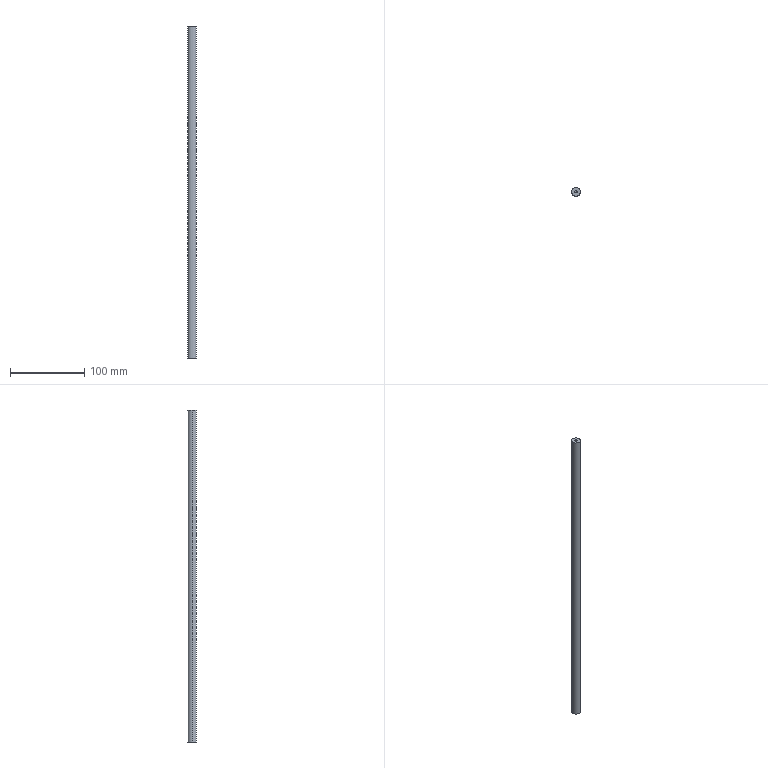Part | SolidWorks | features HoleWzd 2, Extrusion 1 | 1 solid | 12 faces | box 12 x 12 x 448 mm | volume 50405 mm3 | cylinder 6 | cone 4 | plane 2 | commonest cylinder face diameters 3.3 x4 12 x2
STEP:
#1=CARTESIAN_POINT('',(-1.65,0.,433.));
#2=VERTEX_POINT('',#1);
#3=CARTESIAN_POINT('',(1.65,0.,433.));
#4=VERTEX_POINT('',#3);
#5=CARTESIAN_POINT('',(0.,0.,433.));
#6=DIRECTION('',(0.,0.,1.));
#7=DIRECTION('',(1.,0.,0.));
#8=AXIS2_PLACEMENT_3D('',#5,#6,#7);
#9=CIRCLE('',#8,1.65);
#10=EDGE_CURVE('',#2,#4,#9,.T.);
#11=ORIENTED_EDGE('',*,*,#10,.F.);
#12=CARTESIAN_POINT('',(-1.65,0.,448.));
#13=VERTEX_POINT('',#12);
#14=CARTESIAN_POINT('',(-1.65,0.,448.));
#15=DIRECTION('',(0.,0.,1.));
#16=VECTOR('',#15,1000.);
#17=LINE('',#14,#16);
#18=EDGE_CURVE('',#2,#13,#17,.T.);
#19=ORIENTED_EDGE('',*,*,#18,.T.);
#20=CARTESIAN_POINT('',(1.65,0.,448.));
#21=VERTEX_POINT('',#20);
#22=CARTESIAN_POINT('',(0.,0.,448.));
#23=DIRECTION('',(0.,0.,1.));
#24=DIRECTION('',(1.,0.,0.));
#25=AXIS2_PLACEMENT_3D('',#22,#23,#24);
#26=CIRCLE('',#25,1.65);
#27=EDGE_CURVE('',#13,#21,#26,.T.);
#28=ORIENTED_EDGE('',*,*,#27,.T.);
#29=CARTESIAN_POINT('',(1.65,0.,448.));
#30=DIRECTION('',(0.,0.,1.));
#31=VECTOR('',#30,1000.);
#32=LINE('',#29,#31);
#33=EDGE_CURVE('',#4,#21,#32,.T.);
#34=ORIENTED_EDGE('',*,*,#33,.F.);
#35=EDGE_LOOP('',(#11,#19,#28,#34));
#36=FACE_OUTER_BOUND('',#35,.T.);
#37=CARTESIAN_POINT('',(0.,0.,448.));
#38=DIRECTION('',(0.,0.,1.));
#39=DIRECTION('',(1.,0.,0.));
#40=AXIS2_PLACEMENT_3D('',#37,#38,#39);
#41=CYLINDRICAL_SURFACE('',#40,1.65);
#42=ADVANCED_FACE('',(#36),#41,.F.);
#43=CARTESIAN_POINT('',(0.,0.,432.009));
#44=VERTEX_POINT('',#43);
#45=CARTESIAN_POINT('',(1.65,0.,433.));
#46=DIRECTION('',(0.8572,0.,0.515));
#47=VECTOR('',#46,1000.);
#48=LINE('',#45,#47);
#49=EDGE_CURVE('',#44,#4,#48,.T.);
#50=ORIENTED_EDGE('',*,*,#49,.F.);
#51=CARTESIAN_POINT('',(-1.65,0.,433.));
#52=DIRECTION('',(-0.8572,0.,0.515));
#53=VECTOR('',#52,1000.);
#54=LINE('',#51,#53);
#55=EDGE_CURVE('',#44,#2,#54,.T.);
#56=ORIENTED_EDGE('',*,*,#55,.T.);
#57=ORIENTED_EDGE('',*,*,#10,.T.);
#58=EDGE_LOOP('',(#50,#56,#57));
#59=FACE_OUTER_BOUND('',#58,.T.);
#60=CARTESIAN_POINT('',(0.,0.,433.));
#61=DIRECTION('',(0.,0.,1.));
#62=DIRECTION('',(1.,0.,0.));
#63=AXIS2_PLACEMENT_3D('',#60,#61,#62);
#64=CONICAL_SURFACE('',#63,1.65,1.03);
#65=ADVANCED_FACE('',(#59),#64,.F.);
#66=CARTESIAN_POINT('',(1.65,0.,15.));
#67=VERTEX_POINT('',#66);
#68=CARTESIAN_POINT('',(-1.65,0.,15.));
#69=VERTEX_POINT('',#68);
#70=CARTESIAN_POINT('',(0.,0.,15.));
#71=DIRECTION('',(0.,0.,-1.));
#72=DIRECTION('',(-1.,0.,0.));
#73=AXIS2_PLACEMENT_3D('',#70,#71,#72);
#74=CIRCLE('',#73,1.65);
#75=EDGE_CURVE('',#67,#69,#74,.T.);
#76=ORIENTED_EDGE('',*,*,#75,.F.);
#77=CARTESIAN_POINT('',(1.65,0.,0.));
#78=VERTEX_POINT('',#77);
#79=CARTESIAN_POINT('',(1.65,0.,0.));
#80=DIRECTION('',(0.,0.,-1.));
#81=VECTOR('',#80,1000.);
#82=LINE('',#79,#81);
#83=EDGE_CURVE('',#67,#78,#82,.T.);
#84=ORIENTED_EDGE('',*,*,#83,.T.);
#85=CARTESIAN_POINT('',(-1.65,0.,0.));
#86=VERTEX_POINT('',#85);
#87=CARTESIAN_POINT('',(0.,0.,0.));
#88=DIRECTION('',(0.,0.,-1.));
#89=DIRECTION('',(-1.,0.,0.));
#90=AXIS2_PLACEMENT_3D('',#87,#88,#89);
#91=CIRCLE('',#90,1.65);
#92=EDGE_CURVE('',#78,#86,#91,.T.);
#93=ORIENTED_EDGE('',*,*,#92,.T.);
#94=CARTESIAN_POINT('',(-1.65,0.,0.));
#95=DIRECTION('',(0.,0.,-1.));
#96=VECTOR('',#95,1000.);
#97=LINE('',#94,#96);
#98=EDGE_CURVE('',#69,#86,#97,.T.);
#99=ORIENTED_EDGE('',*,*,#98,.F.);
#100=EDGE_LOOP('',(#76,#84,#93,#99));
#101=FACE_OUTER_BOUND('',#100,.T.);
#102=CARTESIAN_POINT('',(0.,0.,0.));
#103=DIRECTION('',(0.,0.,-1.));
#104=DIRECTION('',(-1.,0.,0.));
#105=AXIS2_PLACEMENT_3D('',#102,#103,#104);
#106=CYLINDRICAL_SURFACE('',#105,1.65);
#107=ADVANCED_FACE('',(#101),#106,.F.);
#108=CARTESIAN_POINT('',(0.,0.,15.991));
#109=VERTEX_POINT('',#108);
#110=CARTESIAN_POINT('',(-1.65,0.,15.));
#111=DIRECTION('',(-0.8572,0.,-0.515));
#112=VECTOR('',#111,1000.);
#113=LINE('',#110,#112);
#114=EDGE_CURVE('',#109,#69,#113,.T.);
#115=ORIENTED_EDGE('',*,*,#114,.F.);
#116=CARTESIAN_POINT('',(1.65,0.,15.));
#117=DIRECTION('',(0.8572,0.,-0.515));
#118=VECTOR('',#117,1000.);
#119=LINE('',#116,#118);
#120=EDGE_CURVE('',#109,#67,#119,.T.);
#121=ORIENTED_EDGE('',*,*,#120,.T.);
#122=ORIENTED_EDGE('',*,*,#75,.T.);
#123=EDGE_LOOP('',(#115,#121,#122));
#124=FACE_OUTER_BOUND('',#123,.T.);
#125=CARTESIAN_POINT('',(0.,0.,15.));
#126=DIRECTION('',(0.,0.,-1.));
#127=DIRECTION('',(-1.,0.,0.));
#128=AXIS2_PLACEMENT_3D('',#125,#126,#127);
#129=CONICAL_SURFACE('',#128,1.65,1.03);
#130=ADVANCED_FACE('',(#124),#129,.F.);
#131=CARTESIAN_POINT('',(6.,0.,448.));
#132=VERTEX_POINT('',#131);
#133=CARTESIAN_POINT('',(-6.,0.,448.));
#134=VERTEX_POINT('',#133);
#135=CARTESIAN_POINT('',(0.,0.,448.));
#136=DIRECTION('',(0.,0.,1.));
#137=DIRECTION('',(1.,0.,0.));
#138=AXIS2_PLACEMENT_3D('',#135,#136,#137);
#139=CIRCLE('',#138,6.);
#140=EDGE_CURVE('',#132,#134,#139,.T.);
#141=ORIENTED_EDGE('',*,*,#140,.F.);
#142=CARTESIAN_POINT('',(6.,0.,0.));
#143=VERTEX_POINT('',#142);
#144=CARTESIAN_POINT('',(6.,0.,448.));
#145=DIRECTION('',(0.,0.,-1.));
#146=VECTOR('',#145,1000.);
#147=LINE('',#144,#146);
#148=EDGE_CURVE('',#132,#143,#147,.T.);
#149=ORIENTED_EDGE('',*,*,#148,.T.);
#150=CARTESIAN_POINT('',(-6.,0.,0.));
#151=VERTEX_POINT('',#150);
#152=CARTESIAN_POINT('',(0.,0.,0.));
#153=DIRECTION('',(0.,0.,1.));
#154=DIRECTION('',(1.,0.,0.));
#155=AXIS2_PLACEMENT_3D('',#152,#153,#154);
#156=CIRCLE('',#155,6.);
#157=EDGE_CURVE('',#143,#151,#156,.T.);
#158=ORIENTED_EDGE('',*,*,#157,.T.);
#159=CARTESIAN_POINT('',(-6.,0.,448.));
#160=DIRECTION('',(0.,0.,-1.));
#161=VECTOR('',#160,1000.);
#162=LINE('',#159,#161);
#163=EDGE_CURVE('',#134,#151,#162,.T.);
#164=ORIENTED_EDGE('',*,*,#163,.F.);
#165=EDGE_LOOP('',(#141,#149,#158,#164));
#166=FACE_OUTER_BOUND('',#165,.T.);
#167=CARTESIAN_POINT('',(0.,0.,448.));
#168=DIRECTION('',(0.,0.,-1.));
#169=DIRECTION('',(-1.,0.,0.));
#170=AXIS2_PLACEMENT_3D('',#167,#168,#169);
#171=CYLINDRICAL_SURFACE('',#170,6.);
#172=ADVANCED_FACE('',(#166),#171,.T.);
#173=ORIENTED_EDGE('',*,*,#148,.F.);
#174=CARTESIAN_POINT('',(0.,0.,448.));
#175=DIRECTION('',(0.,0.,1.));
#176=DIRECTION('',(1.,0.,0.));
#177=AXIS2_PLACEMENT_3D('',#174,#175,#176);
#178=CIRCLE('',#177,6.);
#179=EDGE_CURVE('',#134,#132,#178,.T.);
#180=ORIENTED_EDGE('',*,*,#179,.F.);
#181=ORIENTED_EDGE('',*,*,#163,.T.);
#182=CARTESIAN_POINT('',(0.,0.,0.));
#183=DIRECTION('',(0.,0.,1.));
#184=DIRECTION('',(1.,0.,0.));
#185=AXIS2_PLACEMENT_3D('',#182,#183,#184);
#186=CIRCLE('',#185,6.);
#187=EDGE_CURVE('',#151,#143,#186,.T.);
#188=ORIENTED_EDGE('',*,*,#187,.T.);
#189=EDGE_LOOP('',(#173,#180,#181,#188));
#190=FACE_OUTER_BOUND('',#189,.T.);
#191=CARTESIAN_POINT('',(0.,0.,448.));
#192=DIRECTION('',(0.,0.,-1.));
#193=DIRECTION('',(-1.,0.,0.));
#194=AXIS2_PLACEMENT_3D('',#191,#192,#193);
#195=CYLINDRICAL_SURFACE('',#194,6.);
#196=ADVANCED_FACE('',(#190),#195,.T.);
#197=CARTESIAN_POINT('',(0.,0.,448.));
#198=DIRECTION('',(0.,0.,1.));
#199=DIRECTION('',(1.,0.,0.));
#200=AXIS2_PLACEMENT_3D('',#197,#198,#199);
#201=CIRCLE('',#200,1.65);
#202=EDGE_CURVE('',#21,#13,#201,.T.);
#203=ORIENTED_EDGE('',*,*,#202,.F.);
#204=ORIENTED_EDGE('',*,*,#27,.F.);
#205=EDGE_LOOP('',(#203,#204));
#206=FACE_BOUND('',#205,.T.);
#207=ORIENTED_EDGE('',*,*,#179,.T.);
#208=ORIENTED_EDGE('',*,*,#140,.T.);
#209=EDGE_LOOP('',(#207,#208));
#210=FACE_OUTER_BOUND('',#209,.T.);
#211=CARTESIAN_POINT('',(0.,0.,448.));
#212=DIRECTION('',(0.,0.,1.));
#213=DIRECTION('',(1.,0.,0.));
#214=AXIS2_PLACEMENT_3D('',#211,#212,#213);
#215=PLANE('',#214);
#216=ADVANCED_FACE('',(#206,#210),#215,.T.);
#217=CARTESIAN_POINT('',(0.,0.,0.));
#218=DIRECTION('',(0.,0.,-1.));
#219=DIRECTION('',(-1.,0.,0.));
#220=AXIS2_PLACEMENT_3D('',#217,#218,#219);
#221=CIRCLE('',#220,1.65);
#222=EDGE_CURVE('',#86,#78,#221,.T.);
#223=ORIENTED_EDGE('',*,*,#222,.F.);
#224=ORIENTED_EDGE('',*,*,#92,.F.);
#225=EDGE_LOOP('',(#223,#224));
#226=FACE_BOUND('',#225,.T.);
#227=ORIENTED_EDGE('',*,*,#187,.F.);
#228=ORIENTED_EDGE('',*,*,#157,.F.);
#229=EDGE_LOOP('',(#227,#228));
#230=FACE_OUTER_BOUND('',#229,.T.);
#231=CARTESIAN_POINT('',(0.,0.,0.));
#232=DIRECTION('',(0.,0.,1.));
#233=DIRECTION('',(1.,0.,0.));
#234=AXIS2_PLACEMENT_3D('',#231,#232,#233);
#235=PLANE('',#234);
#236=ADVANCED_FACE('',(#226,#230),#235,.F.);
#237=ORIENTED_EDGE('',*,*,#120,.F.);
#238=ORIENTED_EDGE('',*,*,#114,.T.);
#239=CARTESIAN_POINT('',(0.,0.,15.));
#240=DIRECTION('',(0.,0.,-1.));
#241=DIRECTION('',(-1.,0.,0.));
#242=AXIS2_PLACEMENT_3D('',#239,#240,#241);
#243=CIRCLE('',#242,1.65);
#244=EDGE_CURVE('',#69,#67,#243,.T.);
#245=ORIENTED_EDGE('',*,*,#244,.T.);
#246=EDGE_LOOP('',(#237,#238,#245));
#247=FACE_OUTER_BOUND('',#246,.T.);
#248=CARTESIAN_POINT('',(0.,0.,15.));
#249=DIRECTION('',(0.,0.,-1.));
#250=DIRECTION('',(-1.,0.,0.));
#251=AXIS2_PLACEMENT_3D('',#248,#249,#250);
#252=CONICAL_SURFACE('',#251,1.65,1.03);
#253=ADVANCED_FACE('',(#247),#252,.F.);
#254=ORIENTED_EDGE('',*,*,#83,.F.);
#255=ORIENTED_EDGE('',*,*,#244,.F.);
#256=ORIENTED_EDGE('',*,*,#98,.T.);
#257=ORIENTED_EDGE('',*,*,#222,.T.);
#258=EDGE_LOOP('',(#254,#255,#256,#257));
#259=FACE_OUTER_BOUND('',#258,.T.);
#260=CARTESIAN_POINT('',(0.,0.,0.));
#261=DIRECTION('',(0.,0.,-1.));
#262=DIRECTION('',(-1.,0.,0.));
#263=AXIS2_PLACEMENT_3D('',#260,#261,#262);
#264=CYLINDRICAL_SURFACE('',#263,1.65);
#265=ADVANCED_FACE('',(#259),#264,.F.);
#266=ORIENTED_EDGE('',*,*,#55,.F.);
#267=ORIENTED_EDGE('',*,*,#49,.T.);
#268=CARTESIAN_POINT('',(0.,0.,433.));
#269=DIRECTION('',(0.,0.,1.));
#270=DIRECTION('',(1.,0.,0.));
#271=AXIS2_PLACEMENT_3D('',#268,#269,#270);
#272=CIRCLE('',#271,1.65);
#273=EDGE_CURVE('',#4,#2,#272,.T.);
#274=ORIENTED_EDGE('',*,*,#273,.T.);
#275=EDGE_LOOP('',(#266,#267,#274));
#276=FACE_OUTER_BOUND('',#275,.T.);
#277=CARTESIAN_POINT('',(0.,0.,433.));
#278=DIRECTION('',(0.,0.,1.));
#279=DIRECTION('',(1.,0.,0.));
#280=AXIS2_PLACEMENT_3D('',#277,#278,#279);
#281=CONICAL_SURFACE('',#280,1.65,1.03);
#282=ADVANCED_FACE('',(#276),#281,.F.);
#283=ORIENTED_EDGE('',*,*,#18,.F.);
#284=ORIENTED_EDGE('',*,*,#273,.F.);
#285=ORIENTED_EDGE('',*,*,#33,.T.);
#286=ORIENTED_EDGE('',*,*,#202,.T.);
#287=EDGE_LOOP('',(#283,#284,#285,#286));
#288=FACE_OUTER_BOUND('',#287,.T.);
#289=CARTESIAN_POINT('',(0.,0.,448.));
#290=DIRECTION('',(0.,0.,1.));
#291=DIRECTION('',(1.,0.,0.));
#292=AXIS2_PLACEMENT_3D('',#289,#290,#291);
#293=CYLINDRICAL_SURFACE('',#292,1.65);
#294=ADVANCED_FACE('',(#288),#293,.F.);
#295=CLOSED_SHELL('',(#42,#65,#107,#130,#172,#196,#216,#236,#253,#265,#282,#294));
#296=MANIFOLD_SOLID_BREP('',#295);
#297=CARTESIAN_POINT('',(0.,0.,0.));
#298=DIRECTION('',(0.,0.,1.));
#299=DIRECTION('',(1.,0.,0.));
#300=AXIS2_PLACEMENT_3D('',#297,#298,#299);
#301=(LENGTH_UNIT()NAMED_UNIT(*)SI_UNIT(.MILLI.,.METRE.));
#302=UNCERTAINTY_MEASURE_WITH_UNIT(LENGTH_MEASURE(0.00001),#301,'','');
#303=(NAMED_UNIT(*)PLANE_ANGLE_UNIT()SI_UNIT($,.RADIAN.));
#304=(NAMED_UNIT(*)SI_UNIT($,.STERADIAN.)SOLID_ANGLE_UNIT());
#305=(GEOMETRIC_REPRESENTATION_CONTEXT(3)GLOBAL_UNCERTAINTY_ASSIGNED_CONTEXT((#302))GLOBAL_UNIT_ASSIGNED_CONTEXT((#301,#303,#304))REPRESENTATION_CONTEXT('',''));
#306=ADVANCED_BREP_SHAPE_REPRESENTATION('',(#296,#300),#305);